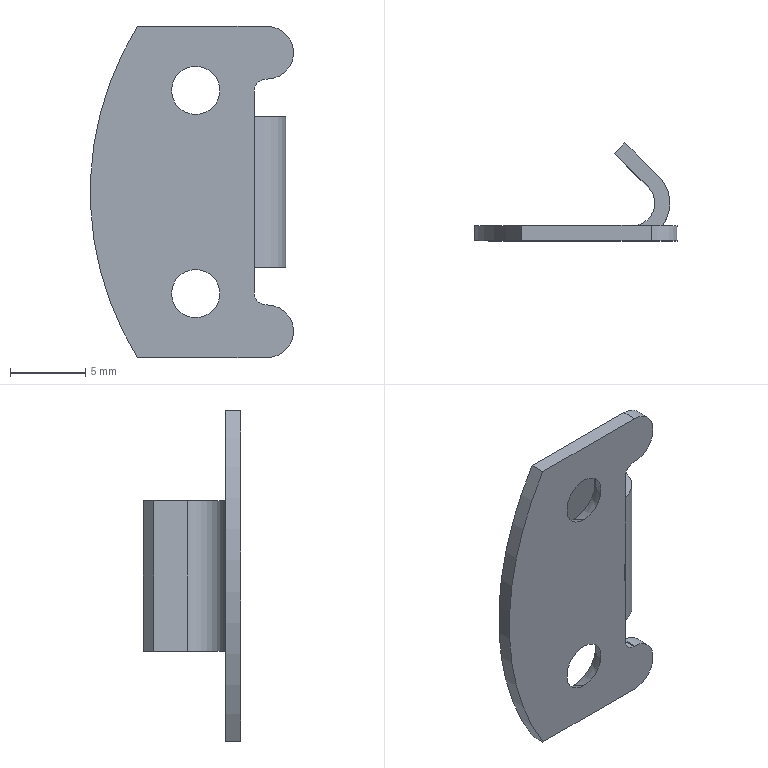Part | SolidWorks | features RefAxis 3, ICE 2, RevCut 2, 3DProfileFeature 1, Extrusion 1 | 1 solid | 23 faces | box 13.5 x 6.5 x 22 mm | volume 286.659 mm3 | plane 12 | cylinder 7 | cone 4 | commonest cylinder face diameters 1.6 x2 3.5 x2 3 x1 5 x1 41.74 x1
STEP:
#1=CARTESIAN_POINT('',(7.,0.,-8.35));
#2=VERTEX_POINT('',#1);
#3=CARTESIAN_POINT('',(7.,0.,-5.15));
#4=VERTEX_POINT('',#3);
#5=CARTESIAN_POINT('',(7.,0.,-6.75));
#6=DIRECTION('',(0.,1.,0.));
#7=DIRECTION('',(0.,0.,1.));
#8=AXIS2_PLACEMENT_3D('',#5,#6,#7);
#9=CIRCLE('',#8,1.6);
#10=EDGE_CURVE('',#2,#4,#9,.T.);
#11=ORIENTED_EDGE('',*,*,#10,.F.);
#12=CARTESIAN_POINT('',(7.,1.,-8.85));
#13=VERTEX_POINT('',#12);
#14=CARTESIAN_POINT('',(7.,0.,-8.35));
#15=DIRECTION('',(0.,0.8944,-0.4472));
#16=VECTOR('',#15,1000.);
#17=LINE('',#14,#16);
#18=EDGE_CURVE('',#2,#13,#17,.T.);
#19=ORIENTED_EDGE('',*,*,#18,.T.);
#20=CARTESIAN_POINT('',(7.,1.,-4.65));
#21=VERTEX_POINT('',#20);
#22=CARTESIAN_POINT('',(7.,1.,-6.75));
#23=DIRECTION('',(0.,1.,0.));
#24=DIRECTION('',(0.,0.,1.));
#25=AXIS2_PLACEMENT_3D('',#22,#23,#24);
#26=CIRCLE('',#25,2.1);
#27=EDGE_CURVE('',#13,#21,#26,.T.);
#28=ORIENTED_EDGE('',*,*,#27,.T.);
#29=CARTESIAN_POINT('',(7.,0.,-5.15));
#30=DIRECTION('',(0.,0.8944,0.4472));
#31=VECTOR('',#30,1000.);
#32=LINE('',#29,#31);
#33=EDGE_CURVE('',#4,#21,#32,.T.);
#34=ORIENTED_EDGE('',*,*,#33,.F.);
#35=EDGE_LOOP('',(#11,#19,#28,#34));
#36=FACE_OUTER_BOUND('',#35,.T.);
#37=CARTESIAN_POINT('',(7.,0.,-6.75));
#38=DIRECTION('',(0.,1.,0.));
#39=DIRECTION('',(0.,0.,1.));
#40=AXIS2_PLACEMENT_3D('',#37,#38,#39);
#41=CONICAL_SURFACE('',#40,1.6,0.4636);
#42=ADVANCED_FACE('',(#36),#41,.F.);
#43=CARTESIAN_POINT('',(7.,0.,5.15));
#44=VERTEX_POINT('',#43);
#45=CARTESIAN_POINT('',(7.,0.,8.35));
#46=VERTEX_POINT('',#45);
#47=CARTESIAN_POINT('',(7.,0.,6.75));
#48=DIRECTION('',(0.,1.,0.));
#49=DIRECTION('',(0.,0.,1.));
#50=AXIS2_PLACEMENT_3D('',#47,#48,#49);
#51=CIRCLE('',#50,1.6);
#52=EDGE_CURVE('',#44,#46,#51,.T.);
#53=ORIENTED_EDGE('',*,*,#52,.F.);
#54=CARTESIAN_POINT('',(7.,1.,4.65));
#55=VERTEX_POINT('',#54);
#56=CARTESIAN_POINT('',(7.,0.,5.15));
#57=DIRECTION('',(0.,0.8944,-0.4472));
#58=VECTOR('',#57,1000.);
#59=LINE('',#56,#58);
#60=EDGE_CURVE('',#44,#55,#59,.T.);
#61=ORIENTED_EDGE('',*,*,#60,.T.);
#62=CARTESIAN_POINT('',(7.,1.,8.85));
#63=VERTEX_POINT('',#62);
#64=CARTESIAN_POINT('',(7.,1.,6.75));
#65=DIRECTION('',(0.,1.,0.));
#66=DIRECTION('',(0.,0.,1.));
#67=AXIS2_PLACEMENT_3D('',#64,#65,#66);
#68=CIRCLE('',#67,2.1);
#69=EDGE_CURVE('',#55,#63,#68,.T.);
#70=ORIENTED_EDGE('',*,*,#69,.T.);
#71=CARTESIAN_POINT('',(7.,0.,8.35));
#72=DIRECTION('',(0.,0.8944,0.4472));
#73=VECTOR('',#72,1000.);
#74=LINE('',#71,#73);
#75=EDGE_CURVE('',#46,#63,#74,.T.);
#76=ORIENTED_EDGE('',*,*,#75,.F.);
#77=EDGE_LOOP('',(#53,#61,#70,#76));
#78=FACE_OUTER_BOUND('',#77,.T.);
#79=CARTESIAN_POINT('',(7.,0.,6.75));
#80=DIRECTION('',(0.,1.,0.));
#81=DIRECTION('',(0.,0.,1.));
#82=AXIS2_PLACEMENT_3D('',#79,#80,#81);
#83=CONICAL_SURFACE('',#82,1.6,0.4636);
#84=ADVANCED_FACE('',(#78),#83,.F.);
#85=CARTESIAN_POINT('',(7.,0.,6.75));
#86=DIRECTION('',(0.,1.,0.));
#87=DIRECTION('',(0.,0.,1.));
#88=AXIS2_PLACEMENT_3D('',#85,#86,#87);
#89=CIRCLE('',#88,1.6);
#90=EDGE_CURVE('',#46,#44,#89,.T.);
#91=ORIENTED_EDGE('',*,*,#90,.T.);
#92=ORIENTED_EDGE('',*,*,#52,.T.);
#93=EDGE_LOOP('',(#91,#92));
#94=FACE_BOUND('',#93,.T.);
#95=CARTESIAN_POINT('',(3.134,0.,11.));
#96=VERTEX_POINT('',#95);
#97=CARTESIAN_POINT('',(11.75,0.,11.));
#98=VERTEX_POINT('',#97);
#99=CARTESIAN_POINT('',(3.134,0.,11.));
#100=DIRECTION('',(1.,0.,0.));
#101=VECTOR('',#100,1000.);
#102=LINE('',#99,#101);
#103=EDGE_CURVE('',#96,#98,#102,.T.);
#104=ORIENTED_EDGE('',*,*,#103,.F.);
#105=CARTESIAN_POINT('',(3.134,0.,-11.));
#106=VERTEX_POINT('',#105);
#107=CARTESIAN_POINT('',(20.87,0.,0.));
#108=DIRECTION('',(0.,1.,0.));
#109=DIRECTION('',(0.,0.,1.));
#110=AXIS2_PLACEMENT_3D('',#107,#108,#109);
#111=CIRCLE('',#110,20.87);
#112=EDGE_CURVE('',#106,#96,#111,.T.);
#113=ORIENTED_EDGE('',*,*,#112,.F.);
#114=CARTESIAN_POINT('',(11.75,0.,-11.));
#115=VERTEX_POINT('',#114);
#116=CARTESIAN_POINT('',(11.75,0.,-11.));
#117=DIRECTION('',(-1.,0.,0.));
#118=VECTOR('',#117,1000.);
#119=LINE('',#116,#118);
#120=EDGE_CURVE('',#115,#106,#119,.T.);
#121=ORIENTED_EDGE('',*,*,#120,.F.);
#122=CARTESIAN_POINT('',(11.75,0.,-7.5));
#123=VERTEX_POINT('',#122);
#124=CARTESIAN_POINT('',(11.75,0.,-9.25));
#125=DIRECTION('',(0.,1.,0.));
#126=DIRECTION('',(0.,0.,1.));
#127=AXIS2_PLACEMENT_3D('',#124,#125,#126);
#128=CIRCLE('',#127,1.75);
#129=EDGE_CURVE('',#123,#115,#128,.T.);
#130=ORIENTED_EDGE('',*,*,#129,.F.);
#131=CARTESIAN_POINT('',(11.69,0.,-7.5));
#132=VERTEX_POINT('',#131);
#133=CARTESIAN_POINT('',(11.69,0.,-7.5));
#134=DIRECTION('',(1.,0.,0.));
#135=VECTOR('',#134,1000.);
#136=LINE('',#133,#135);
#137=EDGE_CURVE('',#132,#123,#136,.T.);
#138=ORIENTED_EDGE('',*,*,#137,.F.);
#139=CARTESIAN_POINT('',(10.89,0.,-6.7));
#140=VERTEX_POINT('',#139);
#141=CARTESIAN_POINT('',(11.69,0.,-6.7));
#142=DIRECTION('',(0.,-1.,0.));
#143=DIRECTION('',(0.,0.,-1.));
#144=AXIS2_PLACEMENT_3D('',#141,#142,#143);
#145=CIRCLE('',#144,0.8);
#146=EDGE_CURVE('',#140,#132,#145,.T.);
#147=ORIENTED_EDGE('',*,*,#146,.F.);
#148=CARTESIAN_POINT('',(10.89,0.,6.7));
#149=VERTEX_POINT('',#148);
#150=CARTESIAN_POINT('',(10.89,0.,6.7));
#151=DIRECTION('',(0.,0.,-1.));
#152=VECTOR('',#151,1000.);
#153=LINE('',#150,#152);
#154=EDGE_CURVE('',#149,#140,#153,.T.);
#155=ORIENTED_EDGE('',*,*,#154,.F.);
#156=CARTESIAN_POINT('',(11.69,0.,7.5));
#157=VERTEX_POINT('',#156);
#158=CARTESIAN_POINT('',(11.69,0.,6.7));
#159=DIRECTION('',(0.,-1.,0.));
#160=DIRECTION('',(0.,0.,-1.));
#161=AXIS2_PLACEMENT_3D('',#158,#159,#160);
#162=CIRCLE('',#161,0.8);
#163=EDGE_CURVE('',#157,#149,#162,.T.);
#164=ORIENTED_EDGE('',*,*,#163,.F.);
#165=CARTESIAN_POINT('',(11.75,0.,7.5));
#166=VERTEX_POINT('',#165);
#167=CARTESIAN_POINT('',(11.75,0.,7.5));
#168=DIRECTION('',(-1.,0.,0.));
#169=VECTOR('',#168,1000.);
#170=LINE('',#167,#169);
#171=EDGE_CURVE('',#166,#157,#170,.T.);
#172=ORIENTED_EDGE('',*,*,#171,.F.);
#173=CARTESIAN_POINT('',(11.75,0.,9.25));
#174=DIRECTION('',(0.,1.,0.));
#175=DIRECTION('',(0.,0.,1.));
#176=AXIS2_PLACEMENT_3D('',#173,#174,#175);
#177=CIRCLE('',#176,1.75);
#178=EDGE_CURVE('',#98,#166,#177,.T.);
#179=ORIENTED_EDGE('',*,*,#178,.F.);
#180=EDGE_LOOP('',(#104,#113,#121,#130,#138,#147,#155,#164,#172,#179));
#181=FACE_OUTER_BOUND('',#180,.T.);
#182=CARTESIAN_POINT('',(7.,0.,-6.75));
#183=DIRECTION('',(0.,1.,0.));
#184=DIRECTION('',(0.,0.,1.));
#185=AXIS2_PLACEMENT_3D('',#182,#183,#184);
#186=CIRCLE('',#185,1.6);
#187=EDGE_CURVE('',#4,#2,#186,.T.);
#188=ORIENTED_EDGE('',*,*,#187,.T.);
#189=ORIENTED_EDGE('',*,*,#10,.T.);
#190=EDGE_LOOP('',(#188,#189));
#191=FACE_BOUND('',#190,.T.);
#192=CARTESIAN_POINT('',(0.,0.,5.));
#193=DIRECTION('',(0.,1.,0.));
#194=DIRECTION('',(0.,0.,1.));
#195=AXIS2_PLACEMENT_3D('',#192,#193,#194);
#196=PLANE('',#195);
#197=ADVANCED_FACE('',(#94,#181,#191),#196,.F.);
#198=CARTESIAN_POINT('',(7.,1.,6.75));
#199=DIRECTION('',(0.,1.,0.));
#200=DIRECTION('',(0.,0.,1.));
#201=AXIS2_PLACEMENT_3D('',#198,#199,#200);
#202=CIRCLE('',#201,2.1);
#203=EDGE_CURVE('',#63,#55,#202,.T.);
#204=ORIENTED_EDGE('',*,*,#203,.F.);
#205=ORIENTED_EDGE('',*,*,#69,.F.);
#206=EDGE_LOOP('',(#204,#205));
#207=FACE_BOUND('',#206,.T.);
#208=CARTESIAN_POINT('',(3.134,1.,-11.));
#209=VERTEX_POINT('',#208);
#210=CARTESIAN_POINT('',(3.134,1.,11.));
#211=VERTEX_POINT('',#210);
#212=CARTESIAN_POINT('',(20.87,1.,0.));
#213=DIRECTION('',(0.,1.,0.));
#214=DIRECTION('',(0.,0.,1.));
#215=AXIS2_PLACEMENT_3D('',#212,#213,#214);
#216=CIRCLE('',#215,20.87);
#217=EDGE_CURVE('',#209,#211,#216,.T.);
#218=ORIENTED_EDGE('',*,*,#217,.T.);
#219=CARTESIAN_POINT('',(11.75,1.,11.));
#220=VERTEX_POINT('',#219);
#221=CARTESIAN_POINT('',(3.134,1.,11.));
#222=DIRECTION('',(1.,0.,0.));
#223=VECTOR('',#222,1000.);
#224=LINE('',#221,#223);
#225=EDGE_CURVE('',#211,#220,#224,.T.);
#226=ORIENTED_EDGE('',*,*,#225,.T.);
#227=CARTESIAN_POINT('',(11.75,1.,7.5));
#228=VERTEX_POINT('',#227);
#229=CARTESIAN_POINT('',(11.75,1.,9.25));
#230=DIRECTION('',(0.,1.,0.));
#231=DIRECTION('',(0.,0.,1.));
#232=AXIS2_PLACEMENT_3D('',#229,#230,#231);
#233=CIRCLE('',#232,1.75);
#234=EDGE_CURVE('',#220,#228,#233,.T.);
#235=ORIENTED_EDGE('',*,*,#234,.T.);
#236=CARTESIAN_POINT('',(11.69,1.,7.5));
#237=VERTEX_POINT('',#236);
#238=CARTESIAN_POINT('',(11.75,1.,7.5));
#239=DIRECTION('',(-1.,0.,0.));
#240=VECTOR('',#239,1000.);
#241=LINE('',#238,#240);
#242=EDGE_CURVE('',#228,#237,#241,.T.);
#243=ORIENTED_EDGE('',*,*,#242,.T.);
#244=CARTESIAN_POINT('',(10.89,1.,6.7));
#245=VERTEX_POINT('',#244);
#246=CARTESIAN_POINT('',(11.69,1.,6.7));
#247=DIRECTION('',(0.,-1.,0.));
#248=DIRECTION('',(0.,0.,-1.));
#249=AXIS2_PLACEMENT_3D('',#246,#247,#248);
#250=CIRCLE('',#249,0.8);
#251=EDGE_CURVE('',#237,#245,#250,.T.);
#252=ORIENTED_EDGE('',*,*,#251,.T.);
#253=CARTESIAN_POINT('',(10.89,1.,5.));
#254=VERTEX_POINT('',#253);
#255=CARTESIAN_POINT('',(10.89,1.,6.7));
#256=DIRECTION('',(0.,0.,-1.));
#257=VECTOR('',#256,1000.);
#258=LINE('',#255,#257);
#259=EDGE_CURVE('',#245,#254,#258,.T.);
#260=ORIENTED_EDGE('',*,*,#259,.T.);
#261=CARTESIAN_POINT('',(10.5,1.,5.));
#262=VERTEX_POINT('',#261);
#263=CARTESIAN_POINT('',(10.5,1.,5.));
#264=DIRECTION('',(-1.,0.,0.));
#265=VECTOR('',#264,1000.);
#266=LINE('',#263,#265);
#267=EDGE_CURVE('',#254,#262,#266,.T.);
#268=ORIENTED_EDGE('',*,*,#267,.T.);
#269=CARTESIAN_POINT('',(10.5,1.,-5.));
#270=VERTEX_POINT('',#269);
#271=CARTESIAN_POINT('',(10.5,1.,5.));
#272=DIRECTION('',(0.,0.,-1.));
#273=VECTOR('',#272,1000.);
#274=LINE('',#271,#273);
#275=EDGE_CURVE('',#262,#270,#274,.T.);
#276=ORIENTED_EDGE('',*,*,#275,.T.);
#277=CARTESIAN_POINT('',(10.89,1.,-5.));
#278=VERTEX_POINT('',#277);
#279=CARTESIAN_POINT('',(10.5,1.,-5.));
#280=DIRECTION('',(-1.,0.,0.));
#281=VECTOR('',#280,1000.);
#282=LINE('',#279,#281);
#283=EDGE_CURVE('',#278,#270,#282,.T.);
#284=ORIENTED_EDGE('',*,*,#283,.F.);
#285=CARTESIAN_POINT('',(10.89,1.,-6.7));
#286=VERTEX_POINT('',#285);
#287=CARTESIAN_POINT('',(10.89,1.,6.7));
#288=DIRECTION('',(0.,0.,-1.));
#289=VECTOR('',#288,1000.);
#290=LINE('',#287,#289);
#291=EDGE_CURVE('',#278,#286,#290,.T.);
#292=ORIENTED_EDGE('',*,*,#291,.T.);
#293=CARTESIAN_POINT('',(11.69,1.,-7.5));
#294=VERTEX_POINT('',#293);
#295=CARTESIAN_POINT('',(11.69,1.,-6.7));
#296=DIRECTION('',(0.,-1.,0.));
#297=DIRECTION('',(0.,0.,-1.));
#298=AXIS2_PLACEMENT_3D('',#295,#296,#297);
#299=CIRCLE('',#298,0.8);
#300=EDGE_CURVE('',#286,#294,#299,.T.);
#301=ORIENTED_EDGE('',*,*,#300,.T.);
#302=CARTESIAN_POINT('',(11.75,1.,-7.5));
#303=VERTEX_POINT('',#302);
#304=CARTESIAN_POINT('',(11.69,1.,-7.5));
#305=DIRECTION('',(1.,0.,0.));
#306=VECTOR('',#305,1000.);
#307=LINE('',#304,#306);
#308=EDGE_CURVE('',#294,#303,#307,.T.);
#309=ORIENTED_EDGE('',*,*,#308,.T.);
#310=CARTESIAN_POINT('',(11.75,1.,-11.));
#311=VERTEX_POINT('',#310);
#312=CARTESIAN_POINT('',(11.75,1.,-9.25));
#313=DIRECTION('',(0.,1.,0.));
#314=DIRECTION('',(0.,0.,1.));
#315=AXIS2_PLACEMENT_3D('',#312,#313,#314);
#316=CIRCLE('',#315,1.75);
#317=EDGE_CURVE('',#303,#311,#316,.T.);
#318=ORIENTED_EDGE('',*,*,#317,.T.);
#319=CARTESIAN_POINT('',(11.75,1.,-11.));
#320=DIRECTION('',(-1.,0.,0.));
#321=VECTOR('',#320,1000.);
#322=LINE('',#319,#321);
#323=EDGE_CURVE('',#311,#209,#322,.T.);
#324=ORIENTED_EDGE('',*,*,#323,.T.);
#325=EDGE_LOOP('',(#218,#226,#235,#243,#252,#260,#268,#276,#284,#292,#301,#309,#318,#324));
#326=FACE_OUTER_BOUND('',#325,.T.);
#327=CARTESIAN_POINT('',(7.,1.,-6.75));
#328=DIRECTION('',(0.,1.,0.));
#329=DIRECTION('',(0.,0.,1.));
#330=AXIS2_PLACEMENT_3D('',#327,#328,#329);
#331=CIRCLE('',#330,2.1);
#332=EDGE_CURVE('',#21,#13,#331,.T.);
#333=ORIENTED_EDGE('',*,*,#332,.F.);
#334=ORIENTED_EDGE('',*,*,#27,.F.);
#335=EDGE_LOOP('',(#333,#334));
#336=FACE_BOUND('',#335,.T.);
#337=CARTESIAN_POINT('',(10.5,1.,5.));
#338=DIRECTION('',(0.,-1.,0.));
#339=DIRECTION('',(0.,0.,-1.));
#340=AXIS2_PLACEMENT_3D('',#337,#338,#339);
#341=PLANE('',#340);
#342=ADVANCED_FACE('',(#207,#326,#336),#341,.F.);
#343=CARTESIAN_POINT('',(10.89,0.03061,-5.));
#344=VERTEX_POINT('',#343);
#345=CARTESIAN_POINT('',(10.89,0.03061,5.));
#346=VERTEX_POINT('',#345);
#347=CARTESIAN_POINT('',(10.89,0.03061,5.));
#348=DIRECTION('',(0.,0.,1.));
#349=VECTOR('',#348,1000.);
#350=LINE('',#347,#349);
#351=EDGE_CURVE('',#344,#346,#350,.T.);
#352=ORIENTED_EDGE('',*,*,#351,.F.);
#353=CARTESIAN_POINT('',(12.254,4.282,-5.));
#354=VERTEX_POINT('',#353);
#355=CARTESIAN_POINT('',(10.5,2.5,-5.));
#356=DIRECTION('',(0.,0.,1.));
#357=DIRECTION('',(1.,0.,0.));
#358=AXIS2_PLACEMENT_3D('',#355,#356,#357);
#359=CIRCLE('',#358,2.5);
#360=EDGE_CURVE('',#344,#354,#359,.T.);
#361=ORIENTED_EDGE('',*,*,#360,.T.);
#362=CARTESIAN_POINT('',(12.254,4.282,5.));
#363=VERTEX_POINT('',#362);
#364=CARTESIAN_POINT('',(12.254,4.282,5.));
#365=DIRECTION('',(0.,0.,-1.));
#366=VECTOR('',#365,1000.);
#367=LINE('',#364,#366);
#368=EDGE_CURVE('',#363,#354,#367,.T.);
#369=ORIENTED_EDGE('',*,*,#368,.F.);
#370=CARTESIAN_POINT('',(10.5,2.5,5.));
#371=DIRECTION('',(0.,0.,1.));
#372=DIRECTION('',(1.,0.,0.));
#373=AXIS2_PLACEMENT_3D('',#370,#371,#372);
#374=CIRCLE('',#373,2.5);
#375=EDGE_CURVE('',#346,#363,#374,.T.);
#376=ORIENTED_EDGE('',*,*,#375,.F.);
#377=EDGE_LOOP('',(#352,#361,#369,#376));
#378=FACE_OUTER_BOUND('',#377,.T.);
#379=CARTESIAN_POINT('',(10.5,2.5,5.));
#380=DIRECTION('',(0.,0.,-1.));
#381=DIRECTION('',(-1.,0.,0.));
#382=AXIS2_PLACEMENT_3D('',#379,#380,#381);
#383=CYLINDRICAL_SURFACE('',#382,2.5);
#384=ADVANCED_FACE('',(#378),#383,.T.);
#385=ORIENTED_EDGE('',*,*,#267,.F.);
#386=CARTESIAN_POINT('',(10.89,2.5,5.));
#387=DIRECTION('',(0.,-1.,0.));
#388=VECTOR('',#387,1000.);
#389=LINE('',#386,#388);
#390=EDGE_CURVE('',#254,#346,#389,.T.);
#391=ORIENTED_EDGE('',*,*,#390,.T.);
#392=ORIENTED_EDGE('',*,*,#375,.T.);
#393=CARTESIAN_POINT('',(10.,6.5,5.));
#394=VERTEX_POINT('',#393);
#395=CARTESIAN_POINT('',(12.254,4.282,5.));
#396=DIRECTION('',(-0.7127,0.7015,0.));
#397=VECTOR('',#396,1000.);
#398=LINE('',#395,#397);
#399=EDGE_CURVE('',#363,#394,#398,.T.);
#400=ORIENTED_EDGE('',*,*,#399,.T.);
#401=CARTESIAN_POINT('',(9.299,5.787,5.));
#402=VERTEX_POINT('',#401);
#403=CARTESIAN_POINT('',(10.,6.5,5.));
#404=DIRECTION('',(-0.7015,-0.7127,0.));
#405=VECTOR('',#404,1000.);
#406=LINE('',#403,#405);
#407=EDGE_CURVE('',#394,#402,#406,.T.);
#408=ORIENTED_EDGE('',*,*,#407,.T.);
#409=CARTESIAN_POINT('',(11.552,3.569,5.));
#410=VERTEX_POINT('',#409);
#411=CARTESIAN_POINT('',(9.299,5.787,5.));
#412=DIRECTION('',(0.7127,-0.7015,0.));
#413=VECTOR('',#412,1000.);
#414=LINE('',#411,#413);
#415=EDGE_CURVE('',#402,#410,#414,.T.);
#416=ORIENTED_EDGE('',*,*,#415,.T.);
#417=CARTESIAN_POINT('',(10.5,2.5,5.));
#418=DIRECTION('',(0.,0.,-1.));
#419=DIRECTION('',(-1.,0.,0.));
#420=AXIS2_PLACEMENT_3D('',#417,#418,#419);
#421=CIRCLE('',#420,1.5);
#422=EDGE_CURVE('',#410,#262,#421,.T.);
#423=ORIENTED_EDGE('',*,*,#422,.T.);
#424=EDGE_LOOP('',(#385,#391,#392,#400,#408,#416,#423));
#425=FACE_OUTER_BOUND('',#424,.T.);
#426=CARTESIAN_POINT('',(10.5,2.5,5.));
#427=DIRECTION('',(0.,0.,1.));
#428=DIRECTION('',(1.,0.,0.));
#429=AXIS2_PLACEMENT_3D('',#426,#427,#428);
#430=PLANE('',#429);
#431=ADVANCED_FACE('',(#425),#430,.T.);
#432=CARTESIAN_POINT('',(10.89,2.5,-5.));
#433=DIRECTION('',(0.,-1.,0.));
#434=VECTOR('',#433,1000.);
#435=LINE('',#432,#434);
#436=EDGE_CURVE('',#278,#344,#435,.T.);
#437=ORIENTED_EDGE('',*,*,#436,.F.);
#438=ORIENTED_EDGE('',*,*,#283,.T.);
#439=CARTESIAN_POINT('',(11.552,3.569,-5.));
#440=VERTEX_POINT('',#439);
#441=CARTESIAN_POINT('',(10.5,2.5,-5.));
#442=DIRECTION('',(0.,0.,-1.));
#443=DIRECTION('',(-1.,0.,0.));
#444=AXIS2_PLACEMENT_3D('',#441,#442,#443);
#445=CIRCLE('',#444,1.5);
#446=EDGE_CURVE('',#440,#270,#445,.T.);
#447=ORIENTED_EDGE('',*,*,#446,.F.);
#448=CARTESIAN_POINT('',(9.299,5.787,-5.));
#449=VERTEX_POINT('',#448);
#450=CARTESIAN_POINT('',(9.299,5.787,-5.));
#451=DIRECTION('',(0.7127,-0.7015,0.));
#452=VECTOR('',#451,1000.);
#453=LINE('',#450,#452);
#454=EDGE_CURVE('',#449,#440,#453,.T.);
#455=ORIENTED_EDGE('',*,*,#454,.F.);
#456=CARTESIAN_POINT('',(10.,6.5,-5.));
#457=VERTEX_POINT('',#456);
#458=CARTESIAN_POINT('',(10.,6.5,-5.));
#459=DIRECTION('',(-0.7015,-0.7127,0.));
#460=VECTOR('',#459,1000.);
#461=LINE('',#458,#460);
#462=EDGE_CURVE('',#457,#449,#461,.T.);
#463=ORIENTED_EDGE('',*,*,#462,.F.);
#464=CARTESIAN_POINT('',(12.254,4.282,-5.));
#465=DIRECTION('',(-0.7127,0.7015,0.));
#466=VECTOR('',#465,1000.);
#467=LINE('',#464,#466);
#468=EDGE_CURVE('',#354,#457,#467,.T.);
#469=ORIENTED_EDGE('',*,*,#468,.F.);
#470=ORIENTED_EDGE('',*,*,#360,.F.);
#471=EDGE_LOOP('',(#437,#438,#447,#455,#463,#469,#470));
#472=FACE_OUTER_BOUND('',#471,.T.);
#473=CARTESIAN_POINT('',(10.5,2.5,-5.));
#474=DIRECTION('',(0.,0.,1.));
#475=DIRECTION('',(1.,0.,0.));
#476=AXIS2_PLACEMENT_3D('',#473,#474,#475);
#477=PLANE('',#476);
#478=ADVANCED_FACE('',(#472),#477,.F.);
#479=ORIENTED_EDGE('',*,*,#368,.T.);
#480=ORIENTED_EDGE('',*,*,#468,.T.);
#481=CARTESIAN_POINT('',(10.,6.5,5.));
#482=DIRECTION('',(0.,0.,-1.));
#483=VECTOR('',#482,1000.);
#484=LINE('',#481,#483);
#485=EDGE_CURVE('',#394,#457,#484,.T.);
#486=ORIENTED_EDGE('',*,*,#485,.F.);
#487=ORIENTED_EDGE('',*,*,#399,.F.);
#488=EDGE_LOOP('',(#479,#480,#486,#487));
#489=FACE_OUTER_BOUND('',#488,.T.);
#490=CARTESIAN_POINT('',(12.254,4.282,5.));
#491=DIRECTION('',(-0.7015,-0.7127,0.));
#492=DIRECTION('',(0.7127,-0.7015,0.));
#493=AXIS2_PLACEMENT_3D('',#490,#491,#492);
#494=PLANE('',#493);
#495=ADVANCED_FACE('',(#489),#494,.F.);
#496=ORIENTED_EDGE('',*,*,#485,.T.);
#497=ORIENTED_EDGE('',*,*,#462,.T.);
#498=CARTESIAN_POINT('',(9.299,5.787,5.));
#499=DIRECTION('',(0.,0.,-1.));
#500=VECTOR('',#499,1000.);
#501=LINE('',#498,#500);
#502=EDGE_CURVE('',#402,#449,#501,.T.);
#503=ORIENTED_EDGE('',*,*,#502,.F.);
#504=ORIENTED_EDGE('',*,*,#407,.F.);
#505=EDGE_LOOP('',(#496,#497,#503,#504));
#506=FACE_OUTER_BOUND('',#505,.T.);
#507=CARTESIAN_POINT('',(10.,6.5,5.));
#508=DIRECTION('',(0.7127,-0.7015,0.));
#509=DIRECTION('',(0.7015,0.7127,0.));
#510=AXIS2_PLACEMENT_3D('',#507,#508,#509);
#511=PLANE('',#510);
#512=ADVANCED_FACE('',(#506),#511,.F.);
#513=ORIENTED_EDGE('',*,*,#502,.T.);
#514=ORIENTED_EDGE('',*,*,#454,.T.);
#515=CARTESIAN_POINT('',(11.552,3.569,5.));
#516=DIRECTION('',(0.,0.,-1.));
#517=VECTOR('',#516,1000.);
#518=LINE('',#515,#517);
#519=EDGE_CURVE('',#410,#440,#518,.T.);
#520=ORIENTED_EDGE('',*,*,#519,.F.);
#521=ORIENTED_EDGE('',*,*,#415,.F.);
#522=EDGE_LOOP('',(#513,#514,#520,#521));
#523=FACE_OUTER_BOUND('',#522,.T.);
#524=CARTESIAN_POINT('',(9.299,5.787,5.));
#525=DIRECTION('',(0.7015,0.7127,0.));
#526=DIRECTION('',(-0.7127,0.7015,0.));
#527=AXIS2_PLACEMENT_3D('',#524,#525,#526);
#528=PLANE('',#527);
#529=ADVANCED_FACE('',(#523),#528,.F.);
#530=ORIENTED_EDGE('',*,*,#519,.T.);
#531=ORIENTED_EDGE('',*,*,#446,.T.);
#532=ORIENTED_EDGE('',*,*,#275,.F.);
#533=ORIENTED_EDGE('',*,*,#422,.F.);
#534=EDGE_LOOP('',(#530,#531,#532,#533));
#535=FACE_OUTER_BOUND('',#534,.T.);
#536=CARTESIAN_POINT('',(10.5,2.5,5.));
#537=DIRECTION('',(0.,0.,-1.));
#538=DIRECTION('',(-1.,0.,0.));
#539=AXIS2_PLACEMENT_3D('',#536,#537,#538);
#540=CYLINDRICAL_SURFACE('',#539,1.5);
#541=ADVANCED_FACE('',(#535),#540,.F.);
#542=ORIENTED_EDGE('',*,*,#112,.T.);
#543=CARTESIAN_POINT('',(3.134,1.,11.));
#544=DIRECTION('',(0.,-1.,0.));
#545=VECTOR('',#544,1000.);
#546=LINE('',#543,#545);
#547=EDGE_CURVE('',#211,#96,#546,.T.);
#548=ORIENTED_EDGE('',*,*,#547,.F.);
#549=ORIENTED_EDGE('',*,*,#217,.F.);
#550=CARTESIAN_POINT('',(3.134,1.,-11.));
#551=DIRECTION('',(0.,-1.,0.));
#552=VECTOR('',#551,1000.);
#553=LINE('',#550,#552);
#554=EDGE_CURVE('',#209,#106,#553,.T.);
#555=ORIENTED_EDGE('',*,*,#554,.T.);
#556=EDGE_LOOP('',(#542,#548,#549,#555));
#557=FACE_OUTER_BOUND('',#556,.T.);
#558=CARTESIAN_POINT('',(20.87,1.,0.));
#559=DIRECTION('',(0.,-1.,0.));
#560=DIRECTION('',(0.,0.,-1.));
#561=AXIS2_PLACEMENT_3D('',#558,#559,#560);
#562=CYLINDRICAL_SURFACE('',#561,20.87);
#563=ADVANCED_FACE('',(#557),#562,.T.);
#564=ORIENTED_EDGE('',*,*,#103,.T.);
#565=CARTESIAN_POINT('',(11.75,1.,11.));
#566=DIRECTION('',(0.,-1.,0.));
#567=VECTOR('',#566,1000.);
#568=LINE('',#565,#567);
#569=EDGE_CURVE('',#220,#98,#568,.T.);
#570=ORIENTED_EDGE('',*,*,#569,.F.);
#571=ORIENTED_EDGE('',*,*,#225,.F.);
#572=ORIENTED_EDGE('',*,*,#547,.T.);
#573=EDGE_LOOP('',(#564,#570,#571,#572));
#574=FACE_OUTER_BOUND('',#573,.T.);
#575=CARTESIAN_POINT('',(3.134,1.,11.));
#576=DIRECTION('',(0.,0.,-1.));
#577=DIRECTION('',(-1.,0.,0.));
#578=AXIS2_PLACEMENT_3D('',#575,#576,#577);
#579=PLANE('',#578);
#580=ADVANCED_FACE('',(#574),#579,.F.);
#581=ORIENTED_EDGE('',*,*,#178,.T.);
#582=CARTESIAN_POINT('',(11.75,1.,7.5));
#583=DIRECTION('',(0.,-1.,0.));
#584=VECTOR('',#583,1000.);
#585=LINE('',#582,#584);
#586=EDGE_CURVE('',#228,#166,#585,.T.);
#587=ORIENTED_EDGE('',*,*,#586,.F.);
#588=ORIENTED_EDGE('',*,*,#234,.F.);
#589=ORIENTED_EDGE('',*,*,#569,.T.);
#590=EDGE_LOOP('',(#581,#587,#588,#589));
#591=FACE_OUTER_BOUND('',#590,.T.);
#592=CARTESIAN_POINT('',(11.75,1.,9.25));
#593=DIRECTION('',(0.,-1.,0.));
#594=DIRECTION('',(0.,0.,-1.));
#595=AXIS2_PLACEMENT_3D('',#592,#593,#594);
#596=CYLINDRICAL_SURFACE('',#595,1.75);
#597=ADVANCED_FACE('',(#591),#596,.T.);
#598=ORIENTED_EDGE('',*,*,#171,.T.);
#599=CARTESIAN_POINT('',(11.69,1.,7.5));
#600=DIRECTION('',(0.,-1.,0.));
#601=VECTOR('',#600,1000.);
#602=LINE('',#599,#601);
#603=EDGE_CURVE('',#237,#157,#602,.T.);
#604=ORIENTED_EDGE('',*,*,#603,.F.);
#605=ORIENTED_EDGE('',*,*,#242,.F.);
#606=ORIENTED_EDGE('',*,*,#586,.T.);
#607=EDGE_LOOP('',(#598,#604,#605,#606));
#608=FACE_OUTER_BOUND('',#607,.T.);
#609=CARTESIAN_POINT('',(11.75,1.,7.5));
#610=DIRECTION('',(0.,0.,1.));
#611=DIRECTION('',(1.,0.,0.));
#612=AXIS2_PLACEMENT_3D('',#609,#610,#611);
#613=PLANE('',#612);
#614=ADVANCED_FACE('',(#608),#613,.F.);
#615=ORIENTED_EDGE('',*,*,#163,.T.);
#616=CARTESIAN_POINT('',(10.89,1.,6.7));
#617=DIRECTION('',(0.,-1.,0.));
#618=VECTOR('',#617,1000.);
#619=LINE('',#616,#618);
#620=EDGE_CURVE('',#245,#149,#619,.T.);
#621=ORIENTED_EDGE('',*,*,#620,.F.);
#622=ORIENTED_EDGE('',*,*,#251,.F.);
#623=ORIENTED_EDGE('',*,*,#603,.T.);
#624=EDGE_LOOP('',(#615,#621,#622,#623));
#625=FACE_OUTER_BOUND('',#624,.T.);
#626=CARTESIAN_POINT('',(11.69,1.,6.7));
#627=DIRECTION('',(0.,-1.,0.));
#628=DIRECTION('',(0.,0.,-1.));
#629=AXIS2_PLACEMENT_3D('',#626,#627,#628);
#630=CYLINDRICAL_SURFACE('',#629,0.8);
#631=ADVANCED_FACE('',(#625),#630,.F.);
#632=ORIENTED_EDGE('',*,*,#390,.F.);
#633=ORIENTED_EDGE('',*,*,#259,.F.);
#634=ORIENTED_EDGE('',*,*,#620,.T.);
#635=ORIENTED_EDGE('',*,*,#154,.T.);
#636=CARTESIAN_POINT('',(10.89,1.,-6.7));
#637=DIRECTION('',(0.,-1.,0.));
#638=VECTOR('',#637,1000.);
#639=LINE('',#636,#638);
#640=EDGE_CURVE('',#286,#140,#639,.T.);
#641=ORIENTED_EDGE('',*,*,#640,.F.);
#642=ORIENTED_EDGE('',*,*,#291,.F.);
#643=ORIENTED_EDGE('',*,*,#436,.T.);
#644=ORIENTED_EDGE('',*,*,#351,.T.);
#645=EDGE_LOOP('',(#632,#633,#634,#635,#641,#642,#643,#644));
#646=FACE_OUTER_BOUND('',#645,.T.);
#647=CARTESIAN_POINT('',(10.89,1.,6.7));
#648=DIRECTION('',(-1.,0.,0.));
#649=DIRECTION('',(0.,0.,1.));
#650=AXIS2_PLACEMENT_3D('',#647,#648,#649);
#651=PLANE('',#650);
#652=ADVANCED_FACE('',(#646),#651,.F.);
#653=ORIENTED_EDGE('',*,*,#146,.T.);
#654=CARTESIAN_POINT('',(11.69,1.,-7.5));
#655=DIRECTION('',(0.,-1.,0.));
#656=VECTOR('',#655,1000.);
#657=LINE('',#654,#656);
#658=EDGE_CURVE('',#294,#132,#657,.T.);
#659=ORIENTED_EDGE('',*,*,#658,.F.);
#660=ORIENTED_EDGE('',*,*,#300,.F.);
#661=ORIENTED_EDGE('',*,*,#640,.T.);
#662=EDGE_LOOP('',(#653,#659,#660,#661));
#663=FACE_OUTER_BOUND('',#662,.T.);
#664=CARTESIAN_POINT('',(11.69,1.,-6.7));
#665=DIRECTION('',(0.,-1.,0.));
#666=DIRECTION('',(0.,0.,-1.));
#667=AXIS2_PLACEMENT_3D('',#664,#665,#666);
#668=CYLINDRICAL_SURFACE('',#667,0.8);
#669=ADVANCED_FACE('',(#663),#668,.F.);
#670=ORIENTED_EDGE('',*,*,#137,.T.);
#671=CARTESIAN_POINT('',(11.75,1.,-7.5));
#672=DIRECTION('',(0.,-1.,0.));
#673=VECTOR('',#672,1000.);
#674=LINE('',#671,#673);
#675=EDGE_CURVE('',#303,#123,#674,.T.);
#676=ORIENTED_EDGE('',*,*,#675,.F.);
#677=ORIENTED_EDGE('',*,*,#308,.F.);
#678=ORIENTED_EDGE('',*,*,#658,.T.);
#679=EDGE_LOOP('',(#670,#676,#677,#678));
#680=FACE_OUTER_BOUND('',#679,.T.);
#681=CARTESIAN_POINT('',(11.69,1.,-7.5));
#682=DIRECTION('',(0.,0.,-1.));
#683=DIRECTION('',(-1.,0.,0.));
#684=AXIS2_PLACEMENT_3D('',#681,#682,#683);
#685=PLANE('',#684);
#686=ADVANCED_FACE('',(#680),#685,.F.);
#687=ORIENTED_EDGE('',*,*,#129,.T.);
#688=CARTESIAN_POINT('',(11.75,1.,-11.));
#689=DIRECTION('',(0.,-1.,0.));
#690=VECTOR('',#689,1000.);
#691=LINE('',#688,#690);
#692=EDGE_CURVE('',#311,#115,#691,.T.);
#693=ORIENTED_EDGE('',*,*,#692,.F.);
#694=ORIENTED_EDGE('',*,*,#317,.F.);
#695=ORIENTED_EDGE('',*,*,#675,.T.);
#696=EDGE_LOOP('',(#687,#693,#694,#695));
#697=FACE_OUTER_BOUND('',#696,.T.);
#698=CARTESIAN_POINT('',(11.75,1.,-9.25));
#699=DIRECTION('',(0.,-1.,0.));
#700=DIRECTION('',(0.,0.,-1.));
#701=AXIS2_PLACEMENT_3D('',#698,#699,#700);
#702=CYLINDRICAL_SURFACE('',#701,1.75);
#703=ADVANCED_FACE('',(#697),#702,.T.);
#704=ORIENTED_EDGE('',*,*,#120,.T.);
#705=ORIENTED_EDGE('',*,*,#554,.F.);
#706=ORIENTED_EDGE('',*,*,#323,.F.);
#707=ORIENTED_EDGE('',*,*,#692,.T.);
#708=EDGE_LOOP('',(#704,#705,#706,#707));
#709=FACE_OUTER_BOUND('',#708,.T.);
#710=CARTESIAN_POINT('',(11.75,1.,-11.));
#711=DIRECTION('',(0.,0.,1.));
#712=DIRECTION('',(1.,0.,0.));
#713=AXIS2_PLACEMENT_3D('',#710,#711,#712);
#714=PLANE('',#713);
#715=ADVANCED_FACE('',(#709),#714,.F.);
#716=ORIENTED_EDGE('',*,*,#60,.F.);
#717=ORIENTED_EDGE('',*,*,#90,.F.);
#718=ORIENTED_EDGE('',*,*,#75,.T.);
#719=ORIENTED_EDGE('',*,*,#203,.T.);
#720=EDGE_LOOP('',(#716,#717,#718,#719));
#721=FACE_OUTER_BOUND('',#720,.T.);
#722=CARTESIAN_POINT('',(7.,0.,6.75));
#723=DIRECTION('',(0.,1.,0.));
#724=DIRECTION('',(0.,0.,1.));
#725=AXIS2_PLACEMENT_3D('',#722,#723,#724);
#726=CONICAL_SURFACE('',#725,1.6,0.4636);
#727=ADVANCED_FACE('',(#721),#726,.F.);
#728=ORIENTED_EDGE('',*,*,#18,.F.);
#729=ORIENTED_EDGE('',*,*,#187,.F.);
#730=ORIENTED_EDGE('',*,*,#33,.T.);
#731=ORIENTED_EDGE('',*,*,#332,.T.);
#732=EDGE_LOOP('',(#728,#729,#730,#731));
#733=FACE_OUTER_BOUND('',#732,.T.);
#734=CARTESIAN_POINT('',(7.,0.,-6.75));
#735=DIRECTION('',(0.,1.,0.));
#736=DIRECTION('',(0.,0.,1.));
#737=AXIS2_PLACEMENT_3D('',#734,#735,#736);
#738=CONICAL_SURFACE('',#737,1.6,0.4636);
#739=ADVANCED_FACE('',(#733),#738,.F.);
#740=CLOSED_SHELL('',(#42,#84,#197,#342,#384,#431,#478,#495,#512,#529,#541,#563,#580,#597,#614,#631,#652,#669,#686,#703,#715,#727,#739));
#741=MANIFOLD_SOLID_BREP('',#740);
#742=CARTESIAN_POINT('',(0.,0.,0.));
#743=DIRECTION('',(0.,0.,1.));
#744=DIRECTION('',(1.,0.,0.));
#745=AXIS2_PLACEMENT_3D('',#742,#743,#744);
#746=(LENGTH_UNIT()NAMED_UNIT(*)SI_UNIT(.MILLI.,.METRE.));
#747=UNCERTAINTY_MEASURE_WITH_UNIT(LENGTH_MEASURE(0.00001),#746,'','');
#748=(NAMED_UNIT(*)PLANE_ANGLE_UNIT()SI_UNIT($,.RADIAN.));
#749=(NAMED_UNIT(*)SI_UNIT($,.STERADIAN.)SOLID_ANGLE_UNIT());
#750=(GEOMETRIC_REPRESENTATION_CONTEXT(3)GLOBAL_UNCERTAINTY_ASSIGNED_CONTEXT((#747))GLOBAL_UNIT_ASSIGNED_CONTEXT((#746,#748,#749))REPRESENTATION_CONTEXT('',''));
#751=ADVANCED_BREP_SHAPE_REPRESENTATION('',(#741,#745),#750);